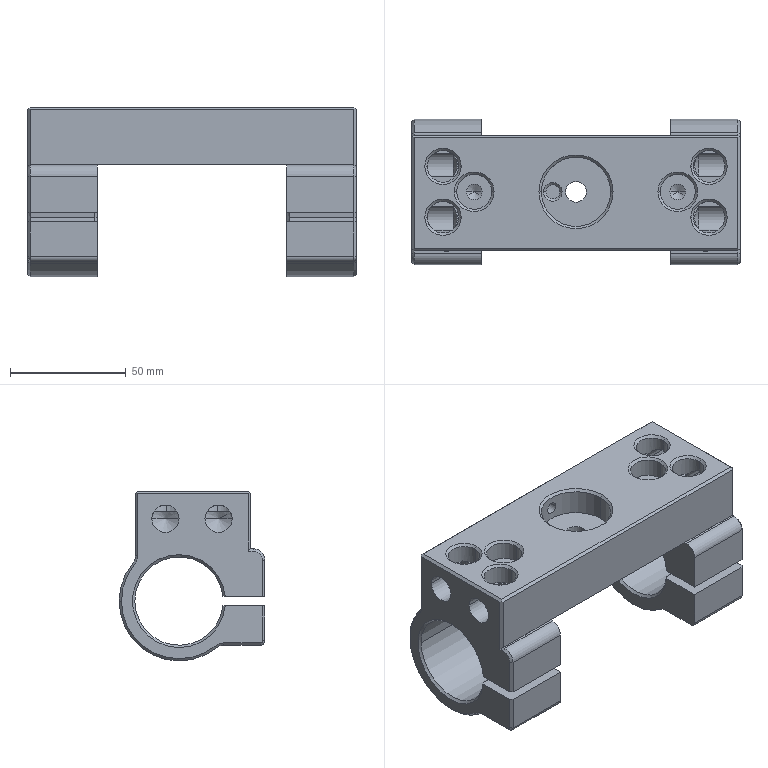Part | 1 solid | 165 faces | box 142 x 63 x 73.5 mm | volume 230284 mm3 | cylinder 62 | cone 53 | plane 50 | commonest cylinder face diameters 6.8 x8 11.8 x8 13.7 x8 9 x6 10 x6 5 x4